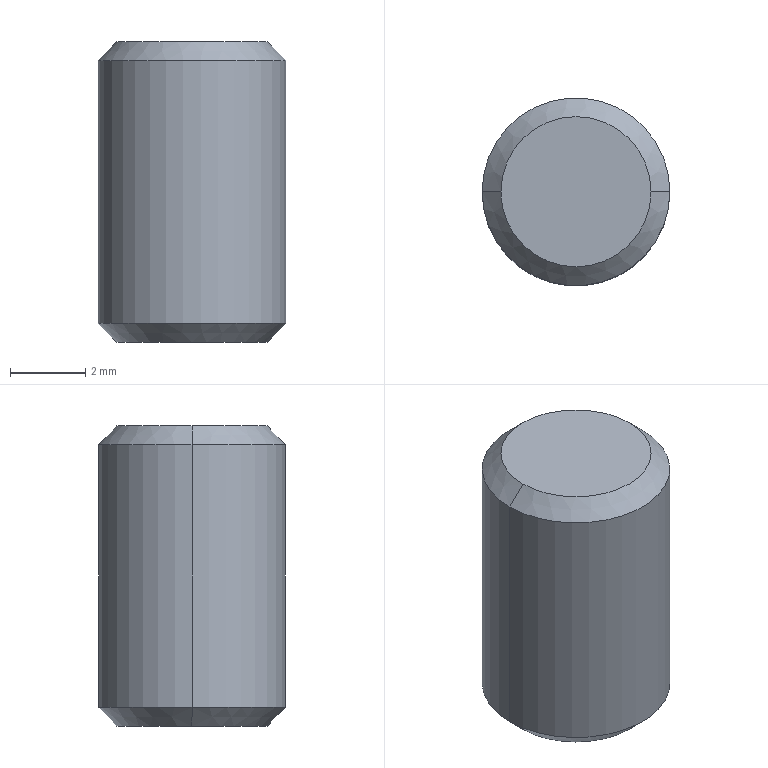Part | SolidWorks | features Revolution 1 | 1 solid | 8 faces | box 5 x 5 x 8 mm | volume 153.414 mm3 | cone 4 | cylinder 2 | plane 2 | commonest cylinder face diameters 5 x2
STEP:
#1=CARTESIAN_POINT('',(-2.,0.,0.));
#2=VERTEX_POINT('',#1);
#3=CARTESIAN_POINT('',(2.,0.,0.));
#4=VERTEX_POINT('',#3);
#5=CARTESIAN_POINT('',(0.,0.,0.));
#6=DIRECTION('',(0.,0.,-1.));
#7=DIRECTION('',(-1.,0.,0.));
#8=AXIS2_PLACEMENT_3D('',#5,#6,#7);
#9=CIRCLE('',#8,2.);
#10=EDGE_CURVE('',#2,#4,#9,.T.);
#11=ORIENTED_EDGE('',*,*,#10,.F.);
#12=CARTESIAN_POINT('',(-2.5,0.,0.5));
#13=VERTEX_POINT('',#12);
#14=CARTESIAN_POINT('',(-2.,0.,0.));
#15=DIRECTION('',(-0.7071,0.,0.7071));
#16=VECTOR('',#15,1000.);
#17=LINE('',#14,#16);
#18=EDGE_CURVE('',#2,#13,#17,.T.);
#19=ORIENTED_EDGE('',*,*,#18,.T.);
#20=CARTESIAN_POINT('',(2.5,0.,0.5));
#21=VERTEX_POINT('',#20);
#22=CARTESIAN_POINT('',(0.,0.,0.5));
#23=DIRECTION('',(0.,0.,-1.));
#24=DIRECTION('',(-1.,0.,0.));
#25=AXIS2_PLACEMENT_3D('',#22,#23,#24);
#26=CIRCLE('',#25,2.5);
#27=EDGE_CURVE('',#13,#21,#26,.T.);
#28=ORIENTED_EDGE('',*,*,#27,.T.);
#29=CARTESIAN_POINT('',(2.,0.,0.));
#30=DIRECTION('',(0.7071,0.,0.7071));
#31=VECTOR('',#30,1000.);
#32=LINE('',#29,#31);
#33=EDGE_CURVE('',#4,#21,#32,.T.);
#34=ORIENTED_EDGE('',*,*,#33,.F.);
#35=EDGE_LOOP('',(#11,#19,#28,#34));
#36=FACE_OUTER_BOUND('',#35,.T.);
#37=CARTESIAN_POINT('',(0.,0.,0.));
#38=DIRECTION('',(0.,0.,1.));
#39=DIRECTION('',(1.,0.,0.));
#40=AXIS2_PLACEMENT_3D('',#37,#38,#39);
#41=CONICAL_SURFACE('',#40,2.,0.7854);
#42=ADVANCED_FACE('',(#36),#41,.T.);
#43=CARTESIAN_POINT('',(-2.5,0.,7.5));
#44=VERTEX_POINT('',#43);
#45=CARTESIAN_POINT('',(2.5,0.,7.5));
#46=VERTEX_POINT('',#45);
#47=CARTESIAN_POINT('',(0.,0.,7.5));
#48=DIRECTION('',(0.,0.,-1.));
#49=DIRECTION('',(-1.,0.,0.));
#50=AXIS2_PLACEMENT_3D('',#47,#48,#49);
#51=CIRCLE('',#50,2.5);
#52=EDGE_CURVE('',#44,#46,#51,.T.);
#53=ORIENTED_EDGE('',*,*,#52,.T.);
#54=CARTESIAN_POINT('',(2.5,0.,8.));
#55=DIRECTION('',(0.,0.,-1.));
#56=VECTOR('',#55,1000.);
#57=LINE('',#54,#56);
#58=EDGE_CURVE('',#46,#21,#57,.T.);
#59=ORIENTED_EDGE('',*,*,#58,.T.);
#60=ORIENTED_EDGE('',*,*,#27,.F.);
#61=CARTESIAN_POINT('',(-2.5,0.,8.));
#62=DIRECTION('',(0.,0.,-1.));
#63=VECTOR('',#62,1000.);
#64=LINE('',#61,#63);
#65=EDGE_CURVE('',#44,#13,#64,.T.);
#66=ORIENTED_EDGE('',*,*,#65,.F.);
#67=EDGE_LOOP('',(#53,#59,#60,#66));
#68=FACE_OUTER_BOUND('',#67,.T.);
#69=CARTESIAN_POINT('',(0.,0.,8.));
#70=DIRECTION('',(0.,0.,-1.));
#71=DIRECTION('',(-1.,0.,0.));
#72=AXIS2_PLACEMENT_3D('',#69,#70,#71);
#73=CYLINDRICAL_SURFACE('',#72,2.5);
#74=ADVANCED_FACE('',(#68),#73,.T.);
#75=CARTESIAN_POINT('',(-2.,0.,8.));
#76=VERTEX_POINT('',#75);
#77=CARTESIAN_POINT('',(2.,0.,8.));
#78=VERTEX_POINT('',#77);
#79=CARTESIAN_POINT('',(0.,0.,8.));
#80=DIRECTION('',(0.,0.,-1.));
#81=DIRECTION('',(-1.,0.,0.));
#82=AXIS2_PLACEMENT_3D('',#79,#80,#81);
#83=CIRCLE('',#82,2.);
#84=EDGE_CURVE('',#76,#78,#83,.T.);
#85=ORIENTED_EDGE('',*,*,#84,.T.);
#86=CARTESIAN_POINT('',(2.5,0.,7.5));
#87=DIRECTION('',(0.7071,0.,-0.7071));
#88=VECTOR('',#87,1000.);
#89=LINE('',#86,#88);
#90=EDGE_CURVE('',#78,#46,#89,.T.);
#91=ORIENTED_EDGE('',*,*,#90,.T.);
#92=ORIENTED_EDGE('',*,*,#52,.F.);
#93=CARTESIAN_POINT('',(-2.5,0.,7.5));
#94=DIRECTION('',(-0.7071,0.,-0.7071));
#95=VECTOR('',#94,1000.);
#96=LINE('',#93,#95);
#97=EDGE_CURVE('',#76,#44,#96,.T.);
#98=ORIENTED_EDGE('',*,*,#97,.F.);
#99=EDGE_LOOP('',(#85,#91,#92,#98));
#100=FACE_OUTER_BOUND('',#99,.T.);
#101=CARTESIAN_POINT('',(0.,0.,7.5));
#102=DIRECTION('',(0.,0.,-1.));
#103=DIRECTION('',(-1.,0.,0.));
#104=AXIS2_PLACEMENT_3D('',#101,#102,#103);
#105=CONICAL_SURFACE('',#104,2.5,0.7854);
#106=ADVANCED_FACE('',(#100),#105,.T.);
#107=ORIENTED_EDGE('',*,*,#90,.F.);
#108=CARTESIAN_POINT('',(0.,0.,8.));
#109=DIRECTION('',(0.,0.,-1.));
#110=DIRECTION('',(-1.,0.,0.));
#111=AXIS2_PLACEMENT_3D('',#108,#109,#110);
#112=CIRCLE('',#111,2.);
#113=EDGE_CURVE('',#78,#76,#112,.T.);
#114=ORIENTED_EDGE('',*,*,#113,.T.);
#115=ORIENTED_EDGE('',*,*,#97,.T.);
#116=CARTESIAN_POINT('',(0.,0.,7.5));
#117=DIRECTION('',(0.,0.,-1.));
#118=DIRECTION('',(-1.,0.,0.));
#119=AXIS2_PLACEMENT_3D('',#116,#117,#118);
#120=CIRCLE('',#119,2.5);
#121=EDGE_CURVE('',#46,#44,#120,.T.);
#122=ORIENTED_EDGE('',*,*,#121,.F.);
#123=EDGE_LOOP('',(#107,#114,#115,#122));
#124=FACE_OUTER_BOUND('',#123,.T.);
#125=CARTESIAN_POINT('',(0.,0.,7.5));
#126=DIRECTION('',(0.,0.,-1.));
#127=DIRECTION('',(-1.,0.,0.));
#128=AXIS2_PLACEMENT_3D('',#125,#126,#127);
#129=CONICAL_SURFACE('',#128,2.5,0.7854);
#130=ADVANCED_FACE('',(#124),#129,.T.);
#131=ORIENTED_EDGE('',*,*,#58,.F.);
#132=ORIENTED_EDGE('',*,*,#121,.T.);
#133=ORIENTED_EDGE('',*,*,#65,.T.);
#134=CARTESIAN_POINT('',(0.,0.,0.5));
#135=DIRECTION('',(0.,0.,-1.));
#136=DIRECTION('',(-1.,0.,0.));
#137=AXIS2_PLACEMENT_3D('',#134,#135,#136);
#138=CIRCLE('',#137,2.5);
#139=EDGE_CURVE('',#21,#13,#138,.T.);
#140=ORIENTED_EDGE('',*,*,#139,.F.);
#141=EDGE_LOOP('',(#131,#132,#133,#140));
#142=FACE_OUTER_BOUND('',#141,.T.);
#143=CARTESIAN_POINT('',(0.,0.,8.));
#144=DIRECTION('',(0.,0.,-1.));
#145=DIRECTION('',(-1.,0.,0.));
#146=AXIS2_PLACEMENT_3D('',#143,#144,#145);
#147=CYLINDRICAL_SURFACE('',#146,2.5);
#148=ADVANCED_FACE('',(#142),#147,.T.);
#149=ORIENTED_EDGE('',*,*,#18,.F.);
#150=CARTESIAN_POINT('',(0.,0.,0.));
#151=DIRECTION('',(0.,0.,-1.));
#152=DIRECTION('',(-1.,0.,0.));
#153=AXIS2_PLACEMENT_3D('',#150,#151,#152);
#154=CIRCLE('',#153,2.);
#155=EDGE_CURVE('',#4,#2,#154,.T.);
#156=ORIENTED_EDGE('',*,*,#155,.F.);
#157=ORIENTED_EDGE('',*,*,#33,.T.);
#158=ORIENTED_EDGE('',*,*,#139,.T.);
#159=EDGE_LOOP('',(#149,#156,#157,#158));
#160=FACE_OUTER_BOUND('',#159,.T.);
#161=CARTESIAN_POINT('',(0.,0.,0.));
#162=DIRECTION('',(0.,0.,1.));
#163=DIRECTION('',(1.,0.,0.));
#164=AXIS2_PLACEMENT_3D('',#161,#162,#163);
#165=CONICAL_SURFACE('',#164,2.,0.7854);
#166=ADVANCED_FACE('',(#160),#165,.T.);
#167=ORIENTED_EDGE('',*,*,#155,.T.);
#168=ORIENTED_EDGE('',*,*,#10,.T.);
#169=EDGE_LOOP('',(#167,#168));
#170=FACE_OUTER_BOUND('',#169,.T.);
#171=CARTESIAN_POINT('',(0.,0.,0.));
#172=DIRECTION('',(0.,0.,-1.));
#173=DIRECTION('',(-1.,0.,0.));
#174=AXIS2_PLACEMENT_3D('',#171,#172,#173);
#175=PLANE('',#174);
#176=ADVANCED_FACE('',(#170),#175,.T.);
#177=ORIENTED_EDGE('',*,*,#84,.F.);
#178=ORIENTED_EDGE('',*,*,#113,.F.);
#179=EDGE_LOOP('',(#177,#178));
#180=FACE_OUTER_BOUND('',#179,.T.);
#181=CARTESIAN_POINT('',(2.,0.,8.));
#182=DIRECTION('',(0.,0.,1.));
#183=DIRECTION('',(1.,0.,0.));
#184=AXIS2_PLACEMENT_3D('',#181,#182,#183);
#185=PLANE('',#184);
#186=ADVANCED_FACE('',(#180),#185,.T.);
#187=CLOSED_SHELL('',(#42,#74,#106,#130,#148,#166,#176,#186));
#188=MANIFOLD_SOLID_BREP('',#187);
#189=CARTESIAN_POINT('',(0.,0.,0.));
#190=DIRECTION('',(0.,0.,1.));
#191=DIRECTION('',(1.,0.,0.));
#192=AXIS2_PLACEMENT_3D('',#189,#190,#191);
#193=(LENGTH_UNIT()NAMED_UNIT(*)SI_UNIT(.MILLI.,.METRE.));
#194=UNCERTAINTY_MEASURE_WITH_UNIT(LENGTH_MEASURE(0.00001),#193,'','');
#195=(NAMED_UNIT(*)PLANE_ANGLE_UNIT()SI_UNIT($,.RADIAN.));
#196=(NAMED_UNIT(*)SI_UNIT($,.STERADIAN.)SOLID_ANGLE_UNIT());
#197=(GEOMETRIC_REPRESENTATION_CONTEXT(3)GLOBAL_UNCERTAINTY_ASSIGNED_CONTEXT((#194))GLOBAL_UNIT_ASSIGNED_CONTEXT((#193,#195,#196))REPRESENTATION_CONTEXT('',''));
#198=ADVANCED_BREP_SHAPE_REPRESENTATION('',(#188,#192),#197);